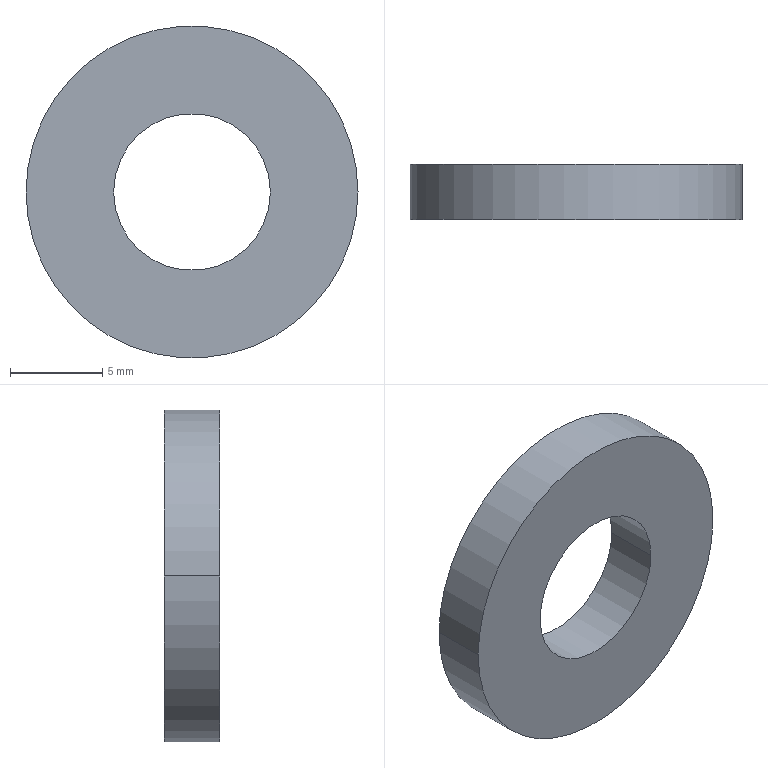Part | STEP file | WSX-SUS-M8X18-3-3 | 1 solid | 6 faces | box 18 x 3 x 18 mm | volume 593.172 mm3 | cylinder 4 | plane 2 | commonest cylinder face diameters 8.5 x2 18 x2
STEP:
#1=CARTESIAN_POINT('',(1.25,0.,0.));
#2=VERTEX_POINT('',#1);
#3=CARTESIAN_POINT('',(-7.25,0.,0.));
#4=VERTEX_POINT('',#3);
#5=CARTESIAN_POINT('',(-3.,0.,0.));
#6=DIRECTION('',(0.,1.,0.));
#7=DIRECTION('',(-1.,0.,0.));
#8=AXIS2_PLACEMENT_3D('',#5,#6,#7);
#9=CIRCLE('',#8,4.25);
#10=EDGE_CURVE('',#2,#4,#9,.T.);
#11=ORIENTED_EDGE('',*,*,#10,.F.);
#12=CARTESIAN_POINT('',(1.25,3.,0.));
#13=VERTEX_POINT('',#12);
#14=CARTESIAN_POINT('',(1.25,0.,0.));
#15=DIRECTION('',(0.,1.,0.));
#16=VECTOR('',#15,1000.);
#17=LINE('',#14,#16);
#18=EDGE_CURVE('',#2,#13,#17,.T.);
#19=ORIENTED_EDGE('',*,*,#18,.T.);
#20=CARTESIAN_POINT('',(-7.25,3.,0.));
#21=VERTEX_POINT('',#20);
#22=CARTESIAN_POINT('',(-3.,3.,0.));
#23=DIRECTION('',(0.,-1.,0.));
#24=DIRECTION('',(1.,0.,0.));
#25=AXIS2_PLACEMENT_3D('',#22,#23,#24);
#26=CIRCLE('',#25,4.25);
#27=EDGE_CURVE('',#21,#13,#26,.T.);
#28=ORIENTED_EDGE('',*,*,#27,.F.);
#29=CARTESIAN_POINT('',(-7.25,0.,0.));
#30=DIRECTION('',(0.,1.,0.));
#31=VECTOR('',#30,1000.);
#32=LINE('',#29,#31);
#33=EDGE_CURVE('',#4,#21,#32,.T.);
#34=ORIENTED_EDGE('',*,*,#33,.F.);
#35=EDGE_LOOP('',(#11,#19,#28,#34));
#36=FACE_OUTER_BOUND('',#35,.T.);
#37=CARTESIAN_POINT('',(-3.,0.,0.));
#38=DIRECTION('',(0.,1.,0.));
#39=DIRECTION('',(-1.,0.,0.));
#40=AXIS2_PLACEMENT_3D('',#37,#38,#39);
#41=CYLINDRICAL_SURFACE('',#40,4.25);
#42=ADVANCED_FACE('',(#36),#41,.F.);
#43=CARTESIAN_POINT('',(-12.,0.,0.));
#44=VERTEX_POINT('',#43);
#45=CARTESIAN_POINT('',(6.,0.,0.));
#46=VERTEX_POINT('',#45);
#47=CARTESIAN_POINT('',(-3.,0.,0.));
#48=DIRECTION('',(0.,1.,0.));
#49=DIRECTION('',(-1.,0.,0.));
#50=AXIS2_PLACEMENT_3D('',#47,#48,#49);
#51=CIRCLE('',#50,9.);
#52=EDGE_CURVE('',#44,#46,#51,.T.);
#53=ORIENTED_EDGE('',*,*,#52,.T.);
#54=CARTESIAN_POINT('',(6.,3.,0.));
#55=VERTEX_POINT('',#54);
#56=CARTESIAN_POINT('',(6.,0.,0.));
#57=DIRECTION('',(0.,1.,0.));
#58=VECTOR('',#57,1000.);
#59=LINE('',#56,#58);
#60=EDGE_CURVE('',#46,#55,#59,.T.);
#61=ORIENTED_EDGE('',*,*,#60,.T.);
#62=CARTESIAN_POINT('',(-12.,3.,0.));
#63=VERTEX_POINT('',#62);
#64=CARTESIAN_POINT('',(-3.,3.,0.));
#65=DIRECTION('',(0.,-1.,0.));
#66=DIRECTION('',(1.,0.,0.));
#67=AXIS2_PLACEMENT_3D('',#64,#65,#66);
#68=CIRCLE('',#67,9.);
#69=EDGE_CURVE('',#55,#63,#68,.T.);
#70=ORIENTED_EDGE('',*,*,#69,.T.);
#71=CARTESIAN_POINT('',(-12.,0.,0.));
#72=DIRECTION('',(0.,1.,0.));
#73=VECTOR('',#72,1000.);
#74=LINE('',#71,#73);
#75=EDGE_CURVE('',#44,#63,#74,.T.);
#76=ORIENTED_EDGE('',*,*,#75,.F.);
#77=EDGE_LOOP('',(#53,#61,#70,#76));
#78=FACE_OUTER_BOUND('',#77,.T.);
#79=CARTESIAN_POINT('',(-3.,0.,0.));
#80=DIRECTION('',(0.,1.,0.));
#81=DIRECTION('',(-1.,0.,0.));
#82=AXIS2_PLACEMENT_3D('',#79,#80,#81);
#83=CYLINDRICAL_SURFACE('',#82,9.);
#84=ADVANCED_FACE('',(#78),#83,.T.);
#85=ORIENTED_EDGE('',*,*,#27,.T.);
#86=CARTESIAN_POINT('',(-3.,3.,0.));
#87=DIRECTION('',(0.,-1.,0.));
#88=DIRECTION('',(1.,0.,0.));
#89=AXIS2_PLACEMENT_3D('',#86,#87,#88);
#90=CIRCLE('',#89,4.25);
#91=EDGE_CURVE('',#13,#21,#90,.T.);
#92=ORIENTED_EDGE('',*,*,#91,.T.);
#93=EDGE_LOOP('',(#85,#92));
#94=FACE_BOUND('',#93,.T.);
#95=CARTESIAN_POINT('',(-3.,3.,0.));
#96=DIRECTION('',(0.,-1.,0.));
#97=DIRECTION('',(1.,0.,0.));
#98=AXIS2_PLACEMENT_3D('',#95,#96,#97);
#99=CIRCLE('',#98,9.);
#100=EDGE_CURVE('',#63,#55,#99,.T.);
#101=ORIENTED_EDGE('',*,*,#100,.F.);
#102=ORIENTED_EDGE('',*,*,#69,.F.);
#103=EDGE_LOOP('',(#101,#102));
#104=FACE_OUTER_BOUND('',#103,.T.);
#105=CARTESIAN_POINT('',(-3.,3.,0.));
#106=DIRECTION('',(0.,1.,0.));
#107=DIRECTION('',(-1.,0.,0.));
#108=AXIS2_PLACEMENT_3D('',#105,#106,#107);
#109=PLANE('',#108);
#110=ADVANCED_FACE('',(#94,#104),#109,.T.);
#111=CARTESIAN_POINT('',(-3.,0.,0.));
#112=DIRECTION('',(0.,1.,0.));
#113=DIRECTION('',(-1.,0.,0.));
#114=AXIS2_PLACEMENT_3D('',#111,#112,#113);
#115=CIRCLE('',#114,4.25);
#116=EDGE_CURVE('',#4,#2,#115,.T.);
#117=ORIENTED_EDGE('',*,*,#116,.T.);
#118=ORIENTED_EDGE('',*,*,#10,.T.);
#119=EDGE_LOOP('',(#117,#118));
#120=FACE_BOUND('',#119,.T.);
#121=ORIENTED_EDGE('',*,*,#52,.F.);
#122=CARTESIAN_POINT('',(-3.,0.,0.));
#123=DIRECTION('',(0.,1.,0.));
#124=DIRECTION('',(-1.,0.,0.));
#125=AXIS2_PLACEMENT_3D('',#122,#123,#124);
#126=CIRCLE('',#125,9.);
#127=EDGE_CURVE('',#46,#44,#126,.T.);
#128=ORIENTED_EDGE('',*,*,#127,.F.);
#129=EDGE_LOOP('',(#121,#128));
#130=FACE_OUTER_BOUND('',#129,.T.);
#131=CARTESIAN_POINT('',(-3.,0.,0.));
#132=DIRECTION('',(0.,-1.,0.));
#133=DIRECTION('',(1.,0.,0.));
#134=AXIS2_PLACEMENT_3D('',#131,#132,#133);
#135=PLANE('',#134);
#136=ADVANCED_FACE('',(#120,#130),#135,.T.);
#137=ORIENTED_EDGE('',*,*,#60,.F.);
#138=ORIENTED_EDGE('',*,*,#127,.T.);
#139=ORIENTED_EDGE('',*,*,#75,.T.);
#140=ORIENTED_EDGE('',*,*,#100,.T.);
#141=EDGE_LOOP('',(#137,#138,#139,#140));
#142=FACE_OUTER_BOUND('',#141,.T.);
#143=CARTESIAN_POINT('',(-3.,0.,0.));
#144=DIRECTION('',(0.,1.,0.));
#145=DIRECTION('',(-1.,0.,0.));
#146=AXIS2_PLACEMENT_3D('',#143,#144,#145);
#147=CYLINDRICAL_SURFACE('',#146,9.);
#148=ADVANCED_FACE('',(#142),#147,.T.);
#149=ORIENTED_EDGE('',*,*,#18,.F.);
#150=ORIENTED_EDGE('',*,*,#116,.F.);
#151=ORIENTED_EDGE('',*,*,#33,.T.);
#152=ORIENTED_EDGE('',*,*,#91,.F.);
#153=EDGE_LOOP('',(#149,#150,#151,#152));
#154=FACE_OUTER_BOUND('',#153,.T.);
#155=CARTESIAN_POINT('',(-3.,0.,0.));
#156=DIRECTION('',(0.,1.,0.));
#157=DIRECTION('',(-1.,0.,0.));
#158=AXIS2_PLACEMENT_3D('',#155,#156,#157);
#159=CYLINDRICAL_SURFACE('',#158,4.25);
#160=ADVANCED_FACE('',(#154),#159,.F.);
#161=CLOSED_SHELL('',(#42,#84,#110,#136,#148,#160));
#162=MANIFOLD_SOLID_BREP('',#161);
#163=CARTESIAN_POINT('',(0.,0.,0.));
#164=DIRECTION('',(0.,0.,1.));
#165=DIRECTION('',(1.,0.,0.));
#166=AXIS2_PLACEMENT_3D('',#163,#164,#165);
#167=(LENGTH_UNIT()NAMED_UNIT(*)SI_UNIT(.MILLI.,.METRE.));
#168=UNCERTAINTY_MEASURE_WITH_UNIT(LENGTH_MEASURE(0.00001),#167,'','');
#169=(NAMED_UNIT(*)PLANE_ANGLE_UNIT()SI_UNIT($,.RADIAN.));
#170=(NAMED_UNIT(*)SI_UNIT($,.STERADIAN.)SOLID_ANGLE_UNIT());
#171=(GEOMETRIC_REPRESENTATION_CONTEXT(3)GLOBAL_UNCERTAINTY_ASSIGNED_CONTEXT((#168))GLOBAL_UNIT_ASSIGNED_CONTEXT((#167,#169,#170))REPRESENTATION_CONTEXT('',''));
#172=ADVANCED_BREP_SHAPE_REPRESENTATION('',(#162,#166),#171);